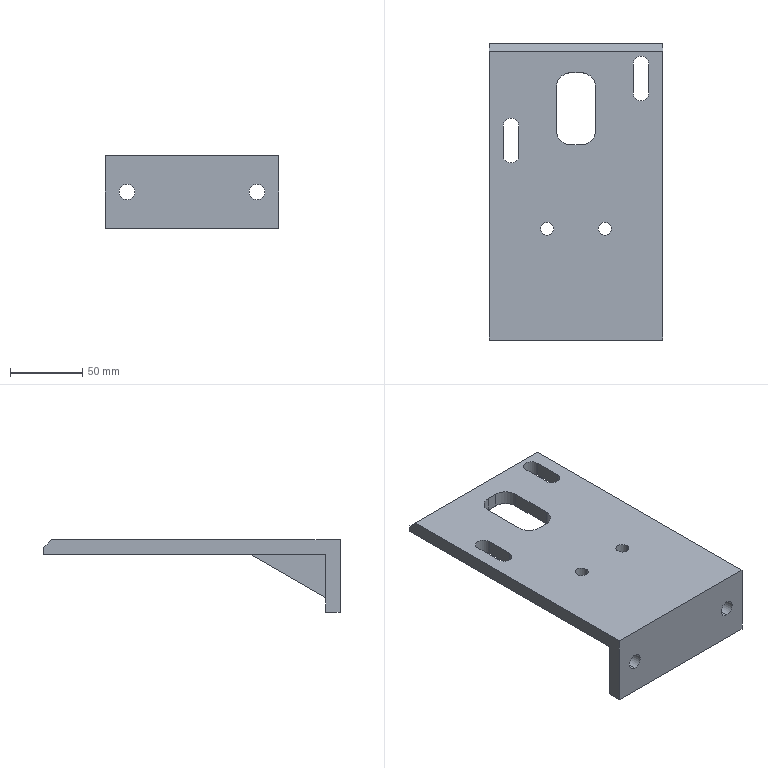Part | 1 solid | 39 faces | box 120 x 205 x 50 mm | volume 285973 mm3 | plane 23 | cylinder 16 | commonest cylinder face diameters 11 x8 9 x4 20 x4
STEP:
#1=CARTESIAN_POINT('',(60.,105.,-5.));
#2=VERTEX_POINT('',#1);
#3=CARTESIAN_POINT('',(60.,100.,0.));
#4=VERTEX_POINT('',#3);
#5=CARTESIAN_POINT('',(60.,100.,0.));
#6=DIRECTION('',(0.,-0.7071,0.7071));
#7=VECTOR('',#6,1000.);
#8=LINE('',#5,#7);
#9=EDGE_CURVE('',#2,#4,#8,.T.);
#10=ORIENTED_EDGE('',*,*,#9,.F.);
#11=CARTESIAN_POINT('',(-60.,105.,-5.));
#12=VERTEX_POINT('',#11);
#13=CARTESIAN_POINT('',(60.,105.,-5.));
#14=DIRECTION('',(1.,0.,0.));
#15=VECTOR('',#14,1000.);
#16=LINE('',#13,#15);
#17=EDGE_CURVE('',#12,#2,#16,.T.);
#18=ORIENTED_EDGE('',*,*,#17,.F.);
#19=CARTESIAN_POINT('',(-60.,100.,0.));
#20=VERTEX_POINT('',#19);
#21=CARTESIAN_POINT('',(-60.,0.,100.));
#22=DIRECTION('',(0.,0.7071,-0.7071));
#23=VECTOR('',#22,1000.);
#24=LINE('',#21,#23);
#25=EDGE_CURVE('',#20,#12,#24,.T.);
#26=ORIENTED_EDGE('',*,*,#25,.F.);
#27=CARTESIAN_POINT('',(60.,100.,0.));
#28=DIRECTION('',(-1.,0.,0.));
#29=VECTOR('',#28,1000.);
#30=LINE('',#27,#29);
#31=EDGE_CURVE('',#4,#20,#30,.T.);
#32=ORIENTED_EDGE('',*,*,#31,.F.);
#33=EDGE_LOOP('',(#10,#18,#26,#32));
#34=FACE_BOUND('',#33,.T.);
#35=CARTESIAN_POINT('',(60.,100.,0.));
#36=DIRECTION('',(0.,-0.7071,-0.7071));
#37=DIRECTION('',(0.,-0.7071,0.7071));
#38=AXIS2_PLACEMENT_3D('',#35,#36,#37);
#39=PLANE('',#38);
#40=ADVANCED_FACE('',(#34),#39,.F.);
#41=CARTESIAN_POINT('',(-15.,-38.038,-10.));
#42=VERTEX_POINT('',#41);
#43=CARTESIAN_POINT('',(-25.,-38.038,-10.));
#44=VERTEX_POINT('',#43);
#45=CARTESIAN_POINT('',(60.,-38.038,-10.));
#46=DIRECTION('',(-1.,0.,0.));
#47=VECTOR('',#46,1000.);
#48=LINE('',#45,#47);
#49=EDGE_CURVE('',#42,#44,#48,.T.);
#50=ORIENTED_EDGE('',*,*,#49,.F.);
#51=CARTESIAN_POINT('',(-15.,-90.,-40.));
#52=VERTEX_POINT('',#51);
#53=CARTESIAN_POINT('',(-15.,-90.,-40.));
#54=DIRECTION('',(0.,0.866,0.5));
#55=VECTOR('',#54,1000.);
#56=LINE('',#53,#55);
#57=EDGE_CURVE('',#52,#42,#56,.T.);
#58=ORIENTED_EDGE('',*,*,#57,.F.);
#59=CARTESIAN_POINT('',(-25.,-90.,-40.));
#60=VERTEX_POINT('',#59);
#61=CARTESIAN_POINT('',(60.,-90.,-40.));
#62=DIRECTION('',(1.,0.,0.));
#63=VECTOR('',#62,1000.);
#64=LINE('',#61,#63);
#65=EDGE_CURVE('',#60,#52,#64,.T.);
#66=ORIENTED_EDGE('',*,*,#65,.F.);
#67=CARTESIAN_POINT('',(-25.,-90.,-40.));
#68=DIRECTION('',(0.,0.866,0.5));
#69=VECTOR('',#68,1000.);
#70=LINE('',#67,#69);
#71=EDGE_CURVE('',#60,#44,#70,.T.);
#72=ORIENTED_EDGE('',*,*,#71,.T.);
#73=EDGE_LOOP('',(#50,#58,#66,#72));
#74=FACE_BOUND('',#73,.T.);
#75=CARTESIAN_POINT('',(-20.,-90.,-40.));
#76=DIRECTION('',(0.,-0.5,0.866));
#77=DIRECTION('',(1.,0.,0.));
#78=AXIS2_PLACEMENT_3D('',#75,#76,#77);
#79=PLANE('',#78);
#80=ADVANCED_FACE('',(#74),#79,.F.);
#81=ORIENTED_EDGE('',*,*,#57,.T.);
#82=CARTESIAN_POINT('',(-15.,-90.,-10.));
#83=VERTEX_POINT('',#82);
#84=CARTESIAN_POINT('',(-15.,-100.,-10.));
#85=DIRECTION('',(0.,-1.,0.));
#86=VECTOR('',#85,1000.);
#87=LINE('',#84,#86);
#88=EDGE_CURVE('',#42,#83,#87,.T.);
#89=ORIENTED_EDGE('',*,*,#88,.T.);
#90=CARTESIAN_POINT('',(-15.,-90.,-50.));
#91=DIRECTION('',(0.,0.,-1.));
#92=VECTOR('',#91,1000.);
#93=LINE('',#90,#92);
#94=EDGE_CURVE('',#83,#52,#93,.T.);
#95=ORIENTED_EDGE('',*,*,#94,.T.);
#96=EDGE_LOOP('',(#81,#89,#95));
#97=FACE_BOUND('',#96,.T.);
#98=CARTESIAN_POINT('',(-15.,2.5,-25.));
#99=DIRECTION('',(-1.,0.,0.));
#100=DIRECTION('',(0.,0.,-1.));
#101=AXIS2_PLACEMENT_3D('',#98,#99,#100);
#102=PLANE('',#101);
#103=ADVANCED_FACE('',(#97),#102,.F.);
#104=CARTESIAN_POINT('',(-25.,-90.,-10.));
#105=VERTEX_POINT('',#104);
#106=CARTESIAN_POINT('',(-25.,-100.,-10.));
#107=DIRECTION('',(0.,-1.,0.));
#108=VECTOR('',#107,1000.);
#109=LINE('',#106,#108);
#110=EDGE_CURVE('',#44,#105,#109,.T.);
#111=ORIENTED_EDGE('',*,*,#110,.F.);
#112=ORIENTED_EDGE('',*,*,#71,.F.);
#113=CARTESIAN_POINT('',(-25.,-90.,-50.));
#114=DIRECTION('',(0.,0.,-1.));
#115=VECTOR('',#114,1000.);
#116=LINE('',#113,#115);
#117=EDGE_CURVE('',#105,#60,#116,.T.);
#118=ORIENTED_EDGE('',*,*,#117,.F.);
#119=EDGE_LOOP('',(#111,#112,#118));
#120=FACE_BOUND('',#119,.T.);
#121=CARTESIAN_POINT('',(-25.,2.5,-25.));
#122=DIRECTION('',(-1.,0.,0.));
#123=DIRECTION('',(0.,0.,-1.));
#124=AXIS2_PLACEMENT_3D('',#121,#122,#123);
#125=PLANE('',#124);
#126=ADVANCED_FACE('',(#120),#125,.T.);
#127=CARTESIAN_POINT('',(25.,-38.038,-10.));
#128=VERTEX_POINT('',#127);
#129=CARTESIAN_POINT('',(15.,-38.038,-10.));
#130=VERTEX_POINT('',#129);
#131=CARTESIAN_POINT('',(60.,-38.038,-10.));
#132=DIRECTION('',(-1.,0.,0.));
#133=VECTOR('',#132,1000.);
#134=LINE('',#131,#133);
#135=EDGE_CURVE('',#128,#130,#134,.T.);
#136=ORIENTED_EDGE('',*,*,#135,.F.);
#137=CARTESIAN_POINT('',(25.,-90.,-40.));
#138=VERTEX_POINT('',#137);
#139=CARTESIAN_POINT('',(25.,-90.,-40.));
#140=DIRECTION('',(0.,0.866,0.5));
#141=VECTOR('',#140,1000.);
#142=LINE('',#139,#141);
#143=EDGE_CURVE('',#138,#128,#142,.T.);
#144=ORIENTED_EDGE('',*,*,#143,.F.);
#145=CARTESIAN_POINT('',(15.,-90.,-40.));
#146=VERTEX_POINT('',#145);
#147=CARTESIAN_POINT('',(60.,-90.,-40.));
#148=DIRECTION('',(1.,0.,0.));
#149=VECTOR('',#148,1000.);
#150=LINE('',#147,#149);
#151=EDGE_CURVE('',#146,#138,#150,.T.);
#152=ORIENTED_EDGE('',*,*,#151,.F.);
#153=CARTESIAN_POINT('',(15.,-90.,-40.));
#154=DIRECTION('',(0.,0.866,0.5));
#155=VECTOR('',#154,1000.);
#156=LINE('',#153,#155);
#157=EDGE_CURVE('',#146,#130,#156,.T.);
#158=ORIENTED_EDGE('',*,*,#157,.T.);
#159=EDGE_LOOP('',(#136,#144,#152,#158));
#160=FACE_BOUND('',#159,.T.);
#161=CARTESIAN_POINT('',(20.,-90.,-40.));
#162=DIRECTION('',(0.,0.5,-0.866));
#163=DIRECTION('',(1.,0.,0.));
#164=AXIS2_PLACEMENT_3D('',#161,#162,#163);
#165=PLANE('',#164);
#166=ADVANCED_FACE('',(#160),#165,.T.);
#167=CARTESIAN_POINT('',(15.,-90.,-10.));
#168=VERTEX_POINT('',#167);
#169=CARTESIAN_POINT('',(15.,-90.,-50.));
#170=DIRECTION('',(0.,0.,1.));
#171=VECTOR('',#170,1000.);
#172=LINE('',#169,#171);
#173=EDGE_CURVE('',#146,#168,#172,.T.);
#174=ORIENTED_EDGE('',*,*,#173,.T.);
#175=CARTESIAN_POINT('',(15.,-100.,-10.));
#176=DIRECTION('',(0.,1.,0.));
#177=VECTOR('',#176,1000.);
#178=LINE('',#175,#177);
#179=EDGE_CURVE('',#168,#130,#178,.T.);
#180=ORIENTED_EDGE('',*,*,#179,.T.);
#181=ORIENTED_EDGE('',*,*,#157,.F.);
#182=EDGE_LOOP('',(#174,#180,#181));
#183=FACE_BOUND('',#182,.T.);
#184=CARTESIAN_POINT('',(15.,2.5,-25.));
#185=DIRECTION('',(1.,0.,0.));
#186=DIRECTION('',(0.,-1.,0.));
#187=AXIS2_PLACEMENT_3D('',#184,#185,#186);
#188=PLANE('',#187);
#189=ADVANCED_FACE('',(#183),#188,.F.);
#190=CARTESIAN_POINT('',(25.,-90.,-10.));
#191=VERTEX_POINT('',#190);
#192=CARTESIAN_POINT('',(25.,-100.,-10.));
#193=DIRECTION('',(0.,1.,0.));
#194=VECTOR('',#193,1000.);
#195=LINE('',#192,#194);
#196=EDGE_CURVE('',#191,#128,#195,.T.);
#197=ORIENTED_EDGE('',*,*,#196,.F.);
#198=CARTESIAN_POINT('',(25.,-90.,-50.));
#199=DIRECTION('',(0.,0.,1.));
#200=VECTOR('',#199,1000.);
#201=LINE('',#198,#200);
#202=EDGE_CURVE('',#138,#191,#201,.T.);
#203=ORIENTED_EDGE('',*,*,#202,.F.);
#204=ORIENTED_EDGE('',*,*,#143,.T.);
#205=EDGE_LOOP('',(#197,#203,#204));
#206=FACE_BOUND('',#205,.T.);
#207=CARTESIAN_POINT('',(25.,2.5,-25.));
#208=DIRECTION('',(1.,0.,0.));
#209=DIRECTION('',(0.,-1.,0.));
#210=AXIS2_PLACEMENT_3D('',#207,#208,#209);
#211=PLANE('',#210);
#212=ADVANCED_FACE('',(#206),#211,.T.);
#213=CARTESIAN_POINT('',(24.5,-23.,0.));
#214=VERTEX_POINT('',#213);
#215=CARTESIAN_POINT('',(24.5,-23.,-10.));
#216=VERTEX_POINT('',#215);
#217=CARTESIAN_POINT('',(24.5,-23.,-10.));
#218=DIRECTION('',(0.,0.,-1.));
#219=VECTOR('',#218,1000.);
#220=LINE('',#217,#219);
#221=EDGE_CURVE('',#214,#216,#220,.T.);
#222=ORIENTED_EDGE('',*,*,#221,.F.);
#223=CARTESIAN_POINT('',(15.5,-23.,0.));
#224=VERTEX_POINT('',#223);
#225=CARTESIAN_POINT('',(20.,-23.,0.));
#226=DIRECTION('',(0.,0.,-1.));
#227=DIRECTION('',(-1.,0.,0.));
#228=AXIS2_PLACEMENT_3D('',#225,#226,#227);
#229=CIRCLE('',#228,4.5);
#230=EDGE_CURVE('',#224,#214,#229,.T.);
#231=ORIENTED_EDGE('',*,*,#230,.F.);
#232=CARTESIAN_POINT('',(15.5,-23.,-10.));
#233=VERTEX_POINT('',#232);
#234=CARTESIAN_POINT('',(15.5,-23.,-10.));
#235=DIRECTION('',(0.,0.,-1.));
#236=VECTOR('',#235,1000.);
#237=LINE('',#234,#236);
#238=EDGE_CURVE('',#224,#233,#237,.T.);
#239=ORIENTED_EDGE('',*,*,#238,.T.);
#240=CARTESIAN_POINT('',(20.,-23.,-10.));
#241=DIRECTION('',(0.,0.,-1.));
#242=DIRECTION('',(-1.,0.,0.));
#243=AXIS2_PLACEMENT_3D('',#240,#241,#242);
#244=CIRCLE('',#243,4.5);
#245=EDGE_CURVE('',#233,#216,#244,.T.);
#246=ORIENTED_EDGE('',*,*,#245,.T.);
#247=EDGE_LOOP('',(#222,#231,#239,#246));
#248=FACE_BOUND('',#247,.T.);
#249=CARTESIAN_POINT('',(20.,-23.,-10.));
#250=DIRECTION('',(0.,0.,-1.));
#251=DIRECTION('',(1.,0.,0.));
#252=AXIS2_PLACEMENT_3D('',#249,#250,#251);
#253=CYLINDRICAL_SURFACE('',#252,4.5);
#254=ADVANCED_FACE('',(#248),#253,.F.);
#255=CARTESIAN_POINT('',(-15.5,-23.,0.));
#256=VERTEX_POINT('',#255);
#257=CARTESIAN_POINT('',(-15.5,-23.,-10.));
#258=VERTEX_POINT('',#257);
#259=CARTESIAN_POINT('',(-15.5,-23.,-10.));
#260=DIRECTION('',(0.,0.,-1.));
#261=VECTOR('',#260,1000.);
#262=LINE('',#259,#261);
#263=EDGE_CURVE('',#256,#258,#262,.T.);
#264=ORIENTED_EDGE('',*,*,#263,.F.);
#265=CARTESIAN_POINT('',(-24.5,-23.,0.));
#266=VERTEX_POINT('',#265);
#267=CARTESIAN_POINT('',(-20.,-23.,0.));
#268=DIRECTION('',(0.,0.,-1.));
#269=DIRECTION('',(-1.,0.,0.));
#270=AXIS2_PLACEMENT_3D('',#267,#268,#269);
#271=CIRCLE('',#270,4.5);
#272=EDGE_CURVE('',#266,#256,#271,.T.);
#273=ORIENTED_EDGE('',*,*,#272,.F.);
#274=CARTESIAN_POINT('',(-24.5,-23.,-10.));
#275=VERTEX_POINT('',#274);
#276=CARTESIAN_POINT('',(-24.5,-23.,-10.));
#277=DIRECTION('',(0.,0.,-1.));
#278=VECTOR('',#277,1000.);
#279=LINE('',#276,#278);
#280=EDGE_CURVE('',#266,#275,#279,.T.);
#281=ORIENTED_EDGE('',*,*,#280,.T.);
#282=CARTESIAN_POINT('',(-20.,-23.,-10.));
#283=DIRECTION('',(0.,0.,-1.));
#284=DIRECTION('',(-1.,0.,0.));
#285=AXIS2_PLACEMENT_3D('',#282,#283,#284);
#286=CIRCLE('',#285,4.5);
#287=EDGE_CURVE('',#275,#258,#286,.T.);
#288=ORIENTED_EDGE('',*,*,#287,.T.);
#289=EDGE_LOOP('',(#264,#273,#281,#288));
#290=FACE_BOUND('',#289,.T.);
#291=CARTESIAN_POINT('',(-20.,-23.,-10.));
#292=DIRECTION('',(0.,0.,-1.));
#293=DIRECTION('',(1.,0.,0.));
#294=AXIS2_PLACEMENT_3D('',#291,#292,#293);
#295=CYLINDRICAL_SURFACE('',#294,4.5);
#296=ADVANCED_FACE('',(#290),#295,.F.);
#297=CARTESIAN_POINT('',(-39.5,48.,-10.));
#298=VERTEX_POINT('',#297);
#299=CARTESIAN_POINT('',(-39.5,28.,-10.));
#300=VERTEX_POINT('',#299);
#301=CARTESIAN_POINT('',(-39.5,48.,-10.));
#302=DIRECTION('',(0.,-1.,0.));
#303=VECTOR('',#302,1000.);
#304=LINE('',#301,#303);
#305=EDGE_CURVE('',#298,#300,#304,.T.);
#306=ORIENTED_EDGE('',*,*,#305,.T.);
#307=CARTESIAN_POINT('',(-39.5,28.,0.));
#308=VERTEX_POINT('',#307);
#309=CARTESIAN_POINT('',(-39.5,28.,0.));
#310=DIRECTION('',(0.,0.,-1.));
#311=VECTOR('',#310,1000.);
#312=LINE('',#309,#311);
#313=EDGE_CURVE('',#308,#300,#312,.T.);
#314=ORIENTED_EDGE('',*,*,#313,.F.);
#315=CARTESIAN_POINT('',(-39.5,48.,0.));
#316=VERTEX_POINT('',#315);
#317=CARTESIAN_POINT('',(-39.5,48.,0.));
#318=DIRECTION('',(0.,-1.,0.));
#319=VECTOR('',#318,1000.);
#320=LINE('',#317,#319);
#321=EDGE_CURVE('',#316,#308,#320,.T.);
#322=ORIENTED_EDGE('',*,*,#321,.F.);
#323=CARTESIAN_POINT('',(-39.5,48.,0.));
#324=DIRECTION('',(0.,0.,-1.));
#325=VECTOR('',#324,1000.);
#326=LINE('',#323,#325);
#327=EDGE_CURVE('',#316,#298,#326,.T.);
#328=ORIENTED_EDGE('',*,*,#327,.T.);
#329=EDGE_LOOP('',(#306,#314,#322,#328));
#330=FACE_BOUND('',#329,.T.);
#331=CARTESIAN_POINT('',(-39.5,48.,0.));
#332=DIRECTION('',(1.,0.,0.));
#333=DIRECTION('',(0.,-1.,0.));
#334=AXIS2_PLACEMENT_3D('',#331,#332,#333);
#335=PLANE('',#334);
#336=ADVANCED_FACE('',(#330),#335,.F.);
#337=CARTESIAN_POINT('',(-50.5,28.,-10.));
#338=VERTEX_POINT('',#337);
#339=CARTESIAN_POINT('',(-45.,28.,-10.));
#340=DIRECTION('',(0.,0.,-1.));
#341=DIRECTION('',(-1.,0.,0.));
#342=AXIS2_PLACEMENT_3D('',#339,#340,#341);
#343=CIRCLE('',#342,5.5);
#344=EDGE_CURVE('',#300,#338,#343,.T.);
#345=ORIENTED_EDGE('',*,*,#344,.T.);
#346=CARTESIAN_POINT('',(-50.5,28.,0.));
#347=VERTEX_POINT('',#346);
#348=CARTESIAN_POINT('',(-50.5,28.,0.));
#349=DIRECTION('',(0.,0.,-1.));
#350=VECTOR('',#349,1000.);
#351=LINE('',#348,#350);
#352=EDGE_CURVE('',#347,#338,#351,.T.);
#353=ORIENTED_EDGE('',*,*,#352,.F.);
#354=CARTESIAN_POINT('',(-45.,28.,0.));
#355=DIRECTION('',(0.,0.,-1.));
#356=DIRECTION('',(-1.,0.,0.));
#357=AXIS2_PLACEMENT_3D('',#354,#355,#356);
#358=CIRCLE('',#357,5.5);
#359=EDGE_CURVE('',#308,#347,#358,.T.);
#360=ORIENTED_EDGE('',*,*,#359,.F.);
#361=ORIENTED_EDGE('',*,*,#313,.T.);
#362=EDGE_LOOP('',(#345,#353,#360,#361));
#363=FACE_BOUND('',#362,.T.);
#364=CARTESIAN_POINT('',(-45.,28.,0.));
#365=DIRECTION('',(0.,0.,-1.));
#366=DIRECTION('',(1.,0.,0.));
#367=AXIS2_PLACEMENT_3D('',#364,#365,#366);
#368=CYLINDRICAL_SURFACE('',#367,5.5);
#369=ADVANCED_FACE('',(#363),#368,.F.);
#370=CARTESIAN_POINT('',(-50.5,48.,-10.));
#371=VERTEX_POINT('',#370);
#372=CARTESIAN_POINT('',(-50.5,48.,-10.));
#373=DIRECTION('',(0.,1.,0.));
#374=VECTOR('',#373,1000.);
#375=LINE('',#372,#374);
#376=EDGE_CURVE('',#338,#371,#375,.T.);
#377=ORIENTED_EDGE('',*,*,#376,.T.);
#378=CARTESIAN_POINT('',(-50.5,48.,0.));
#379=VERTEX_POINT('',#378);
#380=CARTESIAN_POINT('',(-50.5,48.,0.));
#381=DIRECTION('',(0.,0.,-1.));
#382=VECTOR('',#381,1000.);
#383=LINE('',#380,#382);
#384=EDGE_CURVE('',#379,#371,#383,.T.);
#385=ORIENTED_EDGE('',*,*,#384,.F.);
#386=CARTESIAN_POINT('',(-50.5,48.,0.));
#387=DIRECTION('',(0.,1.,0.));
#388=VECTOR('',#387,1000.);
#389=LINE('',#386,#388);
#390=EDGE_CURVE('',#347,#379,#389,.T.);
#391=ORIENTED_EDGE('',*,*,#390,.F.);
#392=ORIENTED_EDGE('',*,*,#352,.T.);
#393=EDGE_LOOP('',(#377,#385,#391,#392));
#394=FACE_BOUND('',#393,.T.);
#395=CARTESIAN_POINT('',(-50.5,48.,0.));
#396=DIRECTION('',(-1.,0.,0.));
#397=DIRECTION('',(0.,0.,-1.));
#398=AXIS2_PLACEMENT_3D('',#395,#396,#397);
#399=PLANE('',#398);
#400=ADVANCED_FACE('',(#394),#399,.F.);
#401=CARTESIAN_POINT('',(-45.,48.,-10.));
#402=DIRECTION('',(0.,0.,-1.));
#403=DIRECTION('',(-1.,0.,0.));
#404=AXIS2_PLACEMENT_3D('',#401,#402,#403);
#405=CIRCLE('',#404,5.5);
#406=EDGE_CURVE('',#371,#298,#405,.T.);
#407=ORIENTED_EDGE('',*,*,#406,.T.);
#408=ORIENTED_EDGE('',*,*,#327,.F.);
#409=CARTESIAN_POINT('',(-45.,48.,0.));
#410=DIRECTION('',(0.,0.,-1.));
#411=DIRECTION('',(-1.,0.,0.));
#412=AXIS2_PLACEMENT_3D('',#409,#410,#411);
#413=CIRCLE('',#412,5.5);
#414=EDGE_CURVE('',#379,#316,#413,.T.);
#415=ORIENTED_EDGE('',*,*,#414,.F.);
#416=ORIENTED_EDGE('',*,*,#384,.T.);
#417=EDGE_LOOP('',(#407,#408,#415,#416));
#418=FACE_BOUND('',#417,.T.);
#419=CARTESIAN_POINT('',(-45.,48.,0.));
#420=DIRECTION('',(0.,0.,-1.));
#421=DIRECTION('',(1.,0.,0.));
#422=AXIS2_PLACEMENT_3D('',#419,#420,#421);
#423=CYLINDRICAL_SURFACE('',#422,5.5);
#424=ADVANCED_FACE('',(#418),#423,.F.);
#425=CARTESIAN_POINT('',(50.5,91.,-10.));
#426=VERTEX_POINT('',#425);
#427=CARTESIAN_POINT('',(50.5,71.,-10.));
#428=VERTEX_POINT('',#427);
#429=CARTESIAN_POINT('',(50.5,91.,-10.));
#430=DIRECTION('',(0.,-1.,0.));
#431=VECTOR('',#430,1000.);
#432=LINE('',#429,#431);
#433=EDGE_CURVE('',#426,#428,#432,.T.);
#434=ORIENTED_EDGE('',*,*,#433,.T.);
#435=CARTESIAN_POINT('',(50.5,71.,0.));
#436=VERTEX_POINT('',#435);
#437=CARTESIAN_POINT('',(50.5,71.,0.));
#438=DIRECTION('',(0.,0.,-1.));
#439=VECTOR('',#438,1000.);
#440=LINE('',#437,#439);
#441=EDGE_CURVE('',#436,#428,#440,.T.);
#442=ORIENTED_EDGE('',*,*,#441,.F.);
#443=CARTESIAN_POINT('',(50.5,91.,0.));
#444=VERTEX_POINT('',#443);
#445=CARTESIAN_POINT('',(50.5,91.,0.));
#446=DIRECTION('',(0.,-1.,0.));
#447=VECTOR('',#446,1000.);
#448=LINE('',#445,#447);
#449=EDGE_CURVE('',#444,#436,#448,.T.);
#450=ORIENTED_EDGE('',*,*,#449,.F.);
#451=CARTESIAN_POINT('',(50.5,91.,0.));
#452=DIRECTION('',(0.,0.,-1.));
#453=VECTOR('',#452,1000.);
#454=LINE('',#451,#453);
#455=EDGE_CURVE('',#444,#426,#454,.T.);
#456=ORIENTED_EDGE('',*,*,#455,.T.);
#457=EDGE_LOOP('',(#434,#442,#450,#456));
#458=FACE_BOUND('',#457,.T.);
#459=CARTESIAN_POINT('',(50.5,91.,0.));
#460=DIRECTION('',(1.,0.,0.));
#461=DIRECTION('',(0.,-1.,0.));
#462=AXIS2_PLACEMENT_3D('',#459,#460,#461);
#463=PLANE('',#462);
#464=ADVANCED_FACE('',(#458),#463,.F.);
#465=CARTESIAN_POINT('',(39.5,71.,-10.));
#466=VERTEX_POINT('',#465);
#467=CARTESIAN_POINT('',(45.,71.,-10.));
#468=DIRECTION('',(0.,0.,-1.));
#469=DIRECTION('',(-1.,0.,0.));
#470=AXIS2_PLACEMENT_3D('',#467,#468,#469);
#471=CIRCLE('',#470,5.5);
#472=EDGE_CURVE('',#428,#466,#471,.T.);
#473=ORIENTED_EDGE('',*,*,#472,.T.);
#474=CARTESIAN_POINT('',(39.5,71.,0.));
#475=VERTEX_POINT('',#474);
#476=CARTESIAN_POINT('',(39.5,71.,0.));
#477=DIRECTION('',(0.,0.,-1.));
#478=VECTOR('',#477,1000.);
#479=LINE('',#476,#478);
#480=EDGE_CURVE('',#475,#466,#479,.T.);
#481=ORIENTED_EDGE('',*,*,#480,.F.);
#482=CARTESIAN_POINT('',(45.,71.,0.));
#483=DIRECTION('',(0.,0.,-1.));
#484=DIRECTION('',(-1.,0.,0.));
#485=AXIS2_PLACEMENT_3D('',#482,#483,#484);
#486=CIRCLE('',#485,5.5);
#487=EDGE_CURVE('',#436,#475,#486,.T.);
#488=ORIENTED_EDGE('',*,*,#487,.F.);
#489=ORIENTED_EDGE('',*,*,#441,.T.);
#490=EDGE_LOOP('',(#473,#481,#488,#489));
#491=FACE_BOUND('',#490,.T.);
#492=CARTESIAN_POINT('',(45.,71.,0.));
#493=DIRECTION('',(0.,0.,-1.));
#494=DIRECTION('',(1.,0.,0.));
#495=AXIS2_PLACEMENT_3D('',#492,#493,#494);
#496=CYLINDRICAL_SURFACE('',#495,5.5);
#497=ADVANCED_FACE('',(#491),#496,.F.);
#498=CARTESIAN_POINT('',(39.5,91.,-10.));
#499=VERTEX_POINT('',#498);
#500=CARTESIAN_POINT('',(39.5,91.,-10.));
#501=DIRECTION('',(0.,1.,0.));
#502=VECTOR('',#501,1000.);
#503=LINE('',#500,#502);
#504=EDGE_CURVE('',#466,#499,#503,.T.);
#505=ORIENTED_EDGE('',*,*,#504,.T.);
#506=CARTESIAN_POINT('',(39.5,91.,0.));
#507=VERTEX_POINT('',#506);
#508=CARTESIAN_POINT('',(39.5,91.,0.));
#509=DIRECTION('',(0.,0.,-1.));
#510=VECTOR('',#509,1000.);
#511=LINE('',#508,#510);
#512=EDGE_CURVE('',#507,#499,#511,.T.);
#513=ORIENTED_EDGE('',*,*,#512,.F.);
#514=CARTESIAN_POINT('',(39.5,91.,0.));
#515=DIRECTION('',(0.,1.,0.));
#516=VECTOR('',#515,1000.);
#517=LINE('',#514,#516);
#518=EDGE_CURVE('',#475,#507,#517,.T.);
#519=ORIENTED_EDGE('',*,*,#518,.F.);
#520=ORIENTED_EDGE('',*,*,#480,.T.);
#521=EDGE_LOOP('',(#505,#513,#519,#520));
#522=FACE_BOUND('',#521,.T.);
#523=CARTESIAN_POINT('',(39.5,91.,0.));
#524=DIRECTION('',(-1.,0.,0.));
#525=DIRECTION('',(0.,0.,-1.));
#526=AXIS2_PLACEMENT_3D('',#523,#524,#525);
#527=PLANE('',#526);
#528=ADVANCED_FACE('',(#522),#527,.F.);
#529=CARTESIAN_POINT('',(45.,91.,-10.));
#530=DIRECTION('',(0.,0.,-1.));
#531=DIRECTION('',(-1.,0.,0.));
#532=AXIS2_PLACEMENT_3D('',#529,#530,#531);
#533=CIRCLE('',#532,5.5);
#534=EDGE_CURVE('',#499,#426,#533,.T.);
#535=ORIENTED_EDGE('',*,*,#534,.T.);
#536=ORIENTED_EDGE('',*,*,#455,.F.);
#537=CARTESIAN_POINT('',(45.,91.,0.));
#538=DIRECTION('',(0.,0.,-1.));
#539=DIRECTION('',(-1.,0.,0.));
#540=AXIS2_PLACEMENT_3D('',#537,#538,#539);
#541=CIRCLE('',#540,5.5);
#542=EDGE_CURVE('',#507,#444,#541,.T.);
#543=ORIENTED_EDGE('',*,*,#542,.F.);
#544=ORIENTED_EDGE('',*,*,#512,.T.);
#545=EDGE_LOOP('',(#535,#536,#543,#544));
#546=FACE_BOUND('',#545,.T.);
#547=CARTESIAN_POINT('',(45.,91.,0.));
#548=DIRECTION('',(0.,0.,-1.));
#549=DIRECTION('',(1.,0.,0.));
#550=AXIS2_PLACEMENT_3D('',#547,#548,#549);
#551=CYLINDRICAL_SURFACE('',#550,5.5);
#552=ADVANCED_FACE('',(#546),#551,.F.);
#553=CARTESIAN_POINT('',(-3.5,35.,0.));
#554=VERTEX_POINT('',#553);
#555=CARTESIAN_POINT('',(-13.5,45.,0.));
#556=VERTEX_POINT('',#555);
#557=CARTESIAN_POINT('',(-3.5,45.,0.));
#558=DIRECTION('',(0.,0.,-1.));
#559=DIRECTION('',(1.,0.,0.));
#560=AXIS2_PLACEMENT_3D('',#557,#558,#559);
#561=CIRCLE('',#560,10.);
#562=EDGE_CURVE('',#554,#556,#561,.T.);
#563=ORIENTED_EDGE('',*,*,#562,.F.);
#564=CARTESIAN_POINT('',(-3.5,35.,-10.));
#565=VERTEX_POINT('',#564);
#566=CARTESIAN_POINT('',(-3.5,35.,0.));
#567=DIRECTION('',(0.,0.,1.));
#568=VECTOR('',#567,1000.);
#569=LINE('',#566,#568);
#570=EDGE_CURVE('',#565,#554,#569,.T.);
#571=ORIENTED_EDGE('',*,*,#570,.F.);
#572=CARTESIAN_POINT('',(-13.5,45.,-10.));
#573=VERTEX_POINT('',#572);
#574=CARTESIAN_POINT('',(-3.5,45.,-10.));
#575=DIRECTION('',(0.,0.,1.));
#576=DIRECTION('',(1.,0.,0.));
#577=AXIS2_PLACEMENT_3D('',#574,#575,#576);
#578=CIRCLE('',#577,10.);
#579=EDGE_CURVE('',#573,#565,#578,.T.);
#580=ORIENTED_EDGE('',*,*,#579,.F.);
#581=CARTESIAN_POINT('',(-13.5,45.,-10.));
#582=DIRECTION('',(0.,0.,-1.));
#583=VECTOR('',#582,1000.);
#584=LINE('',#581,#583);
#585=EDGE_CURVE('',#556,#573,#584,.T.);
#586=ORIENTED_EDGE('',*,*,#585,.F.);
#587=EDGE_LOOP('',(#563,#571,#580,#586));
#588=FACE_BOUND('',#587,.T.);
#589=CARTESIAN_POINT('',(-3.5,45.,0.));
#590=DIRECTION('',(0.,0.,1.));
#591=DIRECTION('',(-1.,0.,0.));
#592=AXIS2_PLACEMENT_3D('',#589,#590,#591);
#593=CYLINDRICAL_SURFACE('',#592,10.);
#594=ADVANCED_FACE('',(#588),#593,.F.);
#595=CARTESIAN_POINT('',(-13.5,75.,0.));
#596=VERTEX_POINT('',#595);
#597=CARTESIAN_POINT('',(-3.5,85.,0.));
#598=VERTEX_POINT('',#597);
#599=CARTESIAN_POINT('',(-3.5,75.,0.));
#600=DIRECTION('',(0.,0.,-1.));
#601=DIRECTION('',(1.,0.,0.));
#602=AXIS2_PLACEMENT_3D('',#599,#600,#601);
#603=CIRCLE('',#602,10.);
#604=EDGE_CURVE('',#596,#598,#603,.T.);
#605=ORIENTED_EDGE('',*,*,#604,.F.);
#606=CARTESIAN_POINT('',(-13.5,75.,-10.));
#607=VERTEX_POINT('',#606);
#608=CARTESIAN_POINT('',(-13.5,75.,0.));
#609=DIRECTION('',(0.,0.,1.));
#610=VECTOR('',#609,1000.);
#611=LINE('',#608,#610);
#612=EDGE_CURVE('',#607,#596,#611,.T.);
#613=ORIENTED_EDGE('',*,*,#612,.F.);
#614=CARTESIAN_POINT('',(-3.5,85.,-10.));
#615=VERTEX_POINT('',#614);
#616=CARTESIAN_POINT('',(-3.5,75.,-10.));
#617=DIRECTION('',(0.,0.,1.));
#618=DIRECTION('',(1.,0.,0.));
#619=AXIS2_PLACEMENT_3D('',#616,#617,#618);
#620=CIRCLE('',#619,10.);
#621=EDGE_CURVE('',#615,#607,#620,.T.);
#622=ORIENTED_EDGE('',*,*,#621,.F.);
#623=CARTESIAN_POINT('',(-3.5,85.,-10.));
#624=DIRECTION('',(0.,0.,-1.));
#625=VECTOR('',#624,1000.);
#626=LINE('',#623,#625);
#627=EDGE_CURVE('',#598,#615,#626,.T.);
#628=ORIENTED_EDGE('',*,*,#627,.F.);
#629=EDGE_LOOP('',(#605,#613,#622,#628));
#630=FACE_BOUND('',#629,.T.);
#631=CARTESIAN_POINT('',(-3.5,75.,0.));
#632=DIRECTION('',(0.,0.,1.));
#633=DIRECTION('',(-1.,0.,0.));
#634=AXIS2_PLACEMENT_3D('',#631,#632,#633);
#635=CYLINDRICAL_SURFACE('',#634,10.);
#636=ADVANCED_FACE('',(#630),#635,.F.);
#637=CARTESIAN_POINT('',(3.5,85.,0.));
#638=VERTEX_POINT('',#637);
#639=CARTESIAN_POINT('',(13.5,75.,0.));
#640=VERTEX_POINT('',#639);
#641=CARTESIAN_POINT('',(3.5,75.,0.));
#642=DIRECTION('',(0.,0.,-1.));
#643=DIRECTION('',(1.,0.,0.));
#644=AXIS2_PLACEMENT_3D('',#641,#642,#643);
#645=CIRCLE('',#644,10.);
#646=EDGE_CURVE('',#638,#640,#645,.T.);
#647=ORIENTED_EDGE('',*,*,#646,.F.);
#648=CARTESIAN_POINT('',(3.5,85.,-10.));
#649=VERTEX_POINT('',#648);
#650=CARTESIAN_POINT('',(3.5,85.,0.));
#651=DIRECTION('',(0.,0.,1.));
#652=VECTOR('',#651,1000.);
#653=LINE('',#650,#652);
#654=EDGE_CURVE('',#649,#638,#653,.T.);
#655=ORIENTED_EDGE('',*,*,#654,.F.);
#656=CARTESIAN_POINT('',(13.5,75.,-10.));
#657=VERTEX_POINT('',#656);
#658=CARTESIAN_POINT('',(3.5,75.,-10.));
#659=DIRECTION('',(0.,0.,1.));
#660=DIRECTION('',(1.,0.,0.));
#661=AXIS2_PLACEMENT_3D('',#658,#659,#660);
#662=CIRCLE('',#661,10.);
#663=EDGE_CURVE('',#657,#649,#662,.T.);
#664=ORIENTED_EDGE('',*,*,#663,.F.);
#665=CARTESIAN_POINT('',(13.5,75.,-10.));
#666=DIRECTION('',(0.,0.,-1.));
#667=VECTOR('',#666,1000.);
#668=LINE('',#665,#667);
#669=EDGE_CURVE('',#640,#657,#668,.T.);
#670=ORIENTED_EDGE('',*,*,#669,.F.);
#671=EDGE_LOOP('',(#647,#655,#664,#670));
#672=FACE_BOUND('',#671,.T.);
#673=CARTESIAN_POINT('',(3.5,75.,0.));
#674=DIRECTION('',(0.,0.,1.));
#675=DIRECTION('',(-1.,0.,0.));
#676=AXIS2_PLACEMENT_3D('',#673,#674,#675);
#677=CYLINDRICAL_SURFACE('',#676,10.);
#678=ADVANCED_FACE('',(#672),#677,.F.);
#679=CARTESIAN_POINT('',(13.5,45.,0.));
#680=VERTEX_POINT('',#679);
#681=CARTESIAN_POINT('',(3.5,35.,0.));
#682=VERTEX_POINT('',#681);
#683=CARTESIAN_POINT('',(3.5,45.,0.));
#684=DIRECTION('',(0.,0.,-1.));
#685=DIRECTION('',(1.,0.,0.));
#686=AXIS2_PLACEMENT_3D('',#683,#684,#685);
#687=CIRCLE('',#686,10.);
#688=EDGE_CURVE('',#680,#682,#687,.T.);
#689=ORIENTED_EDGE('',*,*,#688,.F.);
#690=CARTESIAN_POINT('',(13.5,45.,-10.));
#691=VERTEX_POINT('',#690);
#692=CARTESIAN_POINT('',(13.5,45.,0.));
#693=DIRECTION('',(0.,0.,1.));
#694=VECTOR('',#693,1000.);
#695=LINE('',#692,#694);
#696=EDGE_CURVE('',#691,#680,#695,.T.);
#697=ORIENTED_EDGE('',*,*,#696,.F.);
#698=CARTESIAN_POINT('',(3.5,35.,-10.));
#699=VERTEX_POINT('',#698);
#700=CARTESIAN_POINT('',(3.5,45.,-10.));
#701=DIRECTION('',(0.,0.,1.));
#702=DIRECTION('',(1.,0.,0.));
#703=AXIS2_PLACEMENT_3D('',#700,#701,#702);
#704=CIRCLE('',#703,10.);
#705=EDGE_CURVE('',#699,#691,#704,.T.);
#706=ORIENTED_EDGE('',*,*,#705,.F.);
#707=CARTESIAN_POINT('',(3.5,35.,-10.));
#708=DIRECTION('',(0.,0.,-1.));
#709=VECTOR('',#708,1000.);
#710=LINE('',#707,#709);
#711=EDGE_CURVE('',#682,#699,#710,.T.);
#712=ORIENTED_EDGE('',*,*,#711,.F.);
#713=EDGE_LOOP('',(#689,#697,#706,#712));
#714=FACE_BOUND('',#713,.T.);
#715=CARTESIAN_POINT('',(3.5,45.,0.));
#716=DIRECTION('',(0.,0.,1.));
#717=DIRECTION('',(-1.,0.,0.));
#718=AXIS2_PLACEMENT_3D('',#715,#716,#717);
#719=CYLINDRICAL_SURFACE('',#718,10.);
#720=ADVANCED_FACE('',(#714),#719,.F.);
#721=CARTESIAN_POINT('',(13.5,85.,-10.));
#722=DIRECTION('',(1.,0.,0.));
#723=VECTOR('',#722,1000.);
#724=LINE('',#721,#723);
#725=EDGE_CURVE('',#615,#649,#724,.T.);
#726=ORIENTED_EDGE('',*,*,#725,.T.);
#727=ORIENTED_EDGE('',*,*,#654,.T.);
#728=CARTESIAN_POINT('',(13.5,85.,0.));
#729=DIRECTION('',(1.,0.,0.));
#730=VECTOR('',#729,1000.);
#731=LINE('',#728,#730);
#732=EDGE_CURVE('',#598,#638,#731,.T.);
#733=ORIENTED_EDGE('',*,*,#732,.F.);
#734=ORIENTED_EDGE('',*,*,#627,.T.);
#735=EDGE_LOOP('',(#726,#727,#733,#734));
#736=FACE_BOUND('',#735,.T.);
#737=CARTESIAN_POINT('',(13.5,85.,0.));
#738=DIRECTION('',(0.,1.,0.));
#739=DIRECTION('',(-1.,0.,0.));
#740=AXIS2_PLACEMENT_3D('',#737,#738,#739);
#741=PLANE('',#740);
#742=ADVANCED_FACE('',(#736),#741,.F.);
#743=CARTESIAN_POINT('',(13.5,85.,-10.));
#744=DIRECTION('',(0.,-1.,0.));
#745=VECTOR('',#744,1000.);
#746=LINE('',#743,#745);
#747=EDGE_CURVE('',#657,#691,#746,.T.);
#748=ORIENTED_EDGE('',*,*,#747,.T.);
#749=ORIENTED_EDGE('',*,*,#696,.T.);
#750=CARTESIAN_POINT('',(13.5,85.,0.));
#751=DIRECTION('',(0.,-1.,0.));
#752=VECTOR('',#751,1000.);
#753=LINE('',#750,#752);
#754=EDGE_CURVE('',#640,#680,#753,.T.);
#755=ORIENTED_EDGE('',*,*,#754,.F.);
#756=ORIENTED_EDGE('',*,*,#669,.T.);
#757=EDGE_LOOP('',(#748,#749,#755,#756));
#758=FACE_BOUND('',#757,.T.);
#759=CARTESIAN_POINT('',(13.5,85.,0.));
#760=DIRECTION('',(1.,0.,0.));
#761=DIRECTION('',(0.,-1.,0.));
#762=AXIS2_PLACEMENT_3D('',#759,#760,#761);
#763=PLANE('',#762);
#764=ADVANCED_FACE('',(#758),#763,.F.);
#765=CARTESIAN_POINT('',(13.5,35.,0.));
#766=DIRECTION('',(-1.,0.,0.));
#767=VECTOR('',#766,1000.);
#768=LINE('',#765,#767);
#769=EDGE_CURVE('',#682,#554,#768,.T.);
#770=ORIENTED_EDGE('',*,*,#769,.F.);
#771=ORIENTED_EDGE('',*,*,#711,.T.);
#772=CARTESIAN_POINT('',(13.5,35.,-10.));
#773=DIRECTION('',(-1.,0.,0.));
#774=VECTOR('',#773,1000.);
#775=LINE('',#772,#774);
#776=EDGE_CURVE('',#699,#565,#775,.T.);
#777=ORIENTED_EDGE('',*,*,#776,.T.);
#778=ORIENTED_EDGE('',*,*,#570,.T.);
#779=EDGE_LOOP('',(#770,#771,#777,#778));
#780=FACE_BOUND('',#779,.T.);
#781=CARTESIAN_POINT('',(13.5,35.,0.));
#782=DIRECTION('',(0.,-1.,0.));
#783=DIRECTION('',(0.,0.,1.));
#784=AXIS2_PLACEMENT_3D('',#781,#782,#783);
#785=PLANE('',#784);
#786=ADVANCED_FACE('',(#780),#785,.F.);
#787=CARTESIAN_POINT('',(-13.5,85.,-10.));
#788=DIRECTION('',(0.,1.,0.));
#789=VECTOR('',#788,1000.);
#790=LINE('',#787,#789);
#791=EDGE_CURVE('',#573,#607,#790,.T.);
#792=ORIENTED_EDGE('',*,*,#791,.T.);
#793=ORIENTED_EDGE('',*,*,#612,.T.);
#794=CARTESIAN_POINT('',(-13.5,85.,0.));
#795=DIRECTION('',(0.,1.,0.));
#796=VECTOR('',#795,1000.);
#797=LINE('',#794,#796);
#798=EDGE_CURVE('',#556,#596,#797,.T.);
#799=ORIENTED_EDGE('',*,*,#798,.F.);
#800=ORIENTED_EDGE('',*,*,#585,.T.);
#801=EDGE_LOOP('',(#792,#793,#799,#800));
#802=FACE_BOUND('',#801,.T.);
#803=CARTESIAN_POINT('',(-13.5,85.,0.));
#804=DIRECTION('',(-1.,0.,0.));
#805=DIRECTION('',(0.,0.,-1.));
#806=AXIS2_PLACEMENT_3D('',#803,#804,#805);
#807=PLANE('',#806);
#808=ADVANCED_FACE('',(#802),#807,.F.);
#809=CARTESIAN_POINT('',(-45.,-100.,-30.5));
#810=VERTEX_POINT('',#809);
#811=CARTESIAN_POINT('',(-45.,-90.,-30.5));
#812=VERTEX_POINT('',#811);
#813=CARTESIAN_POINT('',(-45.,-90.,-30.5));
#814=DIRECTION('',(0.,1.,0.));
#815=VECTOR('',#814,1000.);
#816=LINE('',#813,#815);
#817=EDGE_CURVE('',#810,#812,#816,.T.);
#818=ORIENTED_EDGE('',*,*,#817,.F.);
#819=CARTESIAN_POINT('',(-45.,-100.,-19.5));
#820=VERTEX_POINT('',#819);
#821=CARTESIAN_POINT('',(-45.,-100.,-25.));
#822=DIRECTION('',(0.,1.,0.));
#823=DIRECTION('',(0.,0.,1.));
#824=AXIS2_PLACEMENT_3D('',#821,#822,#823);
#825=CIRCLE('',#824,5.5);
#826=EDGE_CURVE('',#820,#810,#825,.T.);
#827=ORIENTED_EDGE('',*,*,#826,.F.);
#828=CARTESIAN_POINT('',(-45.,-90.,-19.5));
#829=VERTEX_POINT('',#828);
#830=CARTESIAN_POINT('',(-45.,-90.,-19.5));
#831=DIRECTION('',(0.,1.,0.));
#832=VECTOR('',#831,1000.);
#833=LINE('',#830,#832);
#834=EDGE_CURVE('',#820,#829,#833,.T.);
#835=ORIENTED_EDGE('',*,*,#834,.T.);
#836=CARTESIAN_POINT('',(-45.,-90.,-25.));
#837=DIRECTION('',(0.,1.,0.));
#838=DIRECTION('',(0.,0.,1.));
#839=AXIS2_PLACEMENT_3D('',#836,#837,#838);
#840=CIRCLE('',#839,5.5);
#841=EDGE_CURVE('',#829,#812,#840,.T.);
#842=ORIENTED_EDGE('',*,*,#841,.T.);
#843=EDGE_LOOP('',(#818,#827,#835,#842));
#844=FACE_BOUND('',#843,.T.);
#845=CARTESIAN_POINT('',(-45.,-90.,-25.));
#846=DIRECTION('',(0.,1.,0.));
#847=DIRECTION('',(0.,0.,-1.));
#848=AXIS2_PLACEMENT_3D('',#845,#846,#847);
#849=CYLINDRICAL_SURFACE('',#848,5.5);
#850=ADVANCED_FACE('',(#844),#849,.F.);
#851=CARTESIAN_POINT('',(45.,-100.,-30.5));
#852=VERTEX_POINT('',#851);
#853=CARTESIAN_POINT('',(45.,-90.,-30.5));
#854=VERTEX_POINT('',#853);
#855=CARTESIAN_POINT('',(45.,-90.,-30.5));
#856=DIRECTION('',(0.,1.,0.));
#857=VECTOR('',#856,1000.);
#858=LINE('',#855,#857);
#859=EDGE_CURVE('',#852,#854,#858,.T.);
#860=ORIENTED_EDGE('',*,*,#859,.F.);
#861=CARTESIAN_POINT('',(45.,-100.,-19.5));
#862=VERTEX_POINT('',#861);
#863=CARTESIAN_POINT('',(45.,-100.,-25.));
#864=DIRECTION('',(0.,1.,0.));
#865=DIRECTION('',(0.,0.,1.));
#866=AXIS2_PLACEMENT_3D('',#863,#864,#865);
#867=CIRCLE('',#866,5.5);
#868=EDGE_CURVE('',#862,#852,#867,.T.);
#869=ORIENTED_EDGE('',*,*,#868,.F.);
#870=CARTESIAN_POINT('',(45.,-90.,-19.5));
#871=VERTEX_POINT('',#870);
#872=CARTESIAN_POINT('',(45.,-90.,-19.5));
#873=DIRECTION('',(0.,1.,0.));
#874=VECTOR('',#873,1000.);
#875=LINE('',#872,#874);
#876=EDGE_CURVE('',#862,#871,#875,.T.);
#877=ORIENTED_EDGE('',*,*,#876,.T.);
#878=CARTESIAN_POINT('',(45.,-90.,-25.));
#879=DIRECTION('',(0.,1.,0.));
#880=DIRECTION('',(0.,0.,1.));
#881=AXIS2_PLACEMENT_3D('',#878,#879,#880);
#882=CIRCLE('',#881,5.5);
#883=EDGE_CURVE('',#871,#854,#882,.T.);
#884=ORIENTED_EDGE('',*,*,#883,.T.);
#885=EDGE_LOOP('',(#860,#869,#877,#884));
#886=FACE_BOUND('',#885,.T.);
#887=CARTESIAN_POINT('',(45.,-90.,-25.));
#888=DIRECTION('',(0.,1.,0.));
#889=DIRECTION('',(0.,0.,-1.));
#890=AXIS2_PLACEMENT_3D('',#887,#888,#889);
#891=CYLINDRICAL_SURFACE('',#890,5.5);
#892=ADVANCED_FACE('',(#886),#891,.F.);
#893=CARTESIAN_POINT('',(-60.,-100.,0.));
#894=VERTEX_POINT('',#893);
#895=CARTESIAN_POINT('',(-60.,-100.,0.));
#896=DIRECTION('',(0.,1.,0.));
#897=VECTOR('',#896,1000.);
#898=LINE('',#895,#897);
#899=EDGE_CURVE('',#894,#20,#898,.T.);
#900=ORIENTED_EDGE('',*,*,#899,.T.);
#901=ORIENTED_EDGE('',*,*,#25,.T.);
#902=CARTESIAN_POINT('',(-60.,105.,-10.));
#903=VERTEX_POINT('',#902);
#904=CARTESIAN_POINT('',(-60.,105.,0.));
#905=DIRECTION('',(0.,0.,-1.));
#906=VECTOR('',#905,1000.);
#907=LINE('',#904,#906);
#908=EDGE_CURVE('',#12,#903,#907,.T.);
#909=ORIENTED_EDGE('',*,*,#908,.T.);
#910=CARTESIAN_POINT('',(-60.,-90.,-10.));
#911=VERTEX_POINT('',#910);
#912=CARTESIAN_POINT('',(-60.,-100.,-10.));
#913=DIRECTION('',(0.,1.,0.));
#914=VECTOR('',#913,1000.);
#915=LINE('',#912,#914);
#916=EDGE_CURVE('',#911,#903,#915,.T.);
#917=ORIENTED_EDGE('',*,*,#916,.F.);
#918=CARTESIAN_POINT('',(-60.,-90.,-50.));
#919=VERTEX_POINT('',#918);
#920=CARTESIAN_POINT('',(-60.,-90.,-50.));
#921=DIRECTION('',(0.,0.,1.));
#922=VECTOR('',#921,1000.);
#923=LINE('',#920,#922);
#924=EDGE_CURVE('',#919,#911,#923,.T.);
#925=ORIENTED_EDGE('',*,*,#924,.F.);
#926=CARTESIAN_POINT('',(-60.,-100.,-50.));
#927=VERTEX_POINT('',#926);
#928=CARTESIAN_POINT('',(-60.,-90.,-50.));
#929=DIRECTION('',(0.,-1.,0.));
#930=VECTOR('',#929,1000.);
#931=LINE('',#928,#930);
#932=EDGE_CURVE('',#919,#927,#931,.T.);
#933=ORIENTED_EDGE('',*,*,#932,.T.);
#934=CARTESIAN_POINT('',(-60.,-100.,-50.));
#935=DIRECTION('',(0.,0.,1.));
#936=VECTOR('',#935,1000.);
#937=LINE('',#934,#936);
#938=EDGE_CURVE('',#927,#894,#937,.T.);
#939=ORIENTED_EDGE('',*,*,#938,.T.);
#940=EDGE_LOOP('',(#900,#901,#909,#917,#925,#933,#939));
#941=FACE_BOUND('',#940,.T.);
#942=CARTESIAN_POINT('',(-60.,-100.,0.));
#943=DIRECTION('',(-1.,0.,0.));
#944=DIRECTION('',(0.,0.,-1.));
#945=AXIS2_PLACEMENT_3D('',#942,#943,#944);
#946=PLANE('',#945);
#947=ADVANCED_FACE('',(#941),#946,.T.);
#948=CARTESIAN_POINT('',(60.,105.,-10.));
#949=VERTEX_POINT('',#948);
#950=CARTESIAN_POINT('',(60.,105.,0.));
#951=DIRECTION('',(0.,0.,-1.));
#952=VECTOR('',#951,1000.);
#953=LINE('',#950,#952);
#954=EDGE_CURVE('',#2,#949,#953,.T.);
#955=ORIENTED_EDGE('',*,*,#954,.F.);
#956=ORIENTED_EDGE('',*,*,#9,.T.);
#957=CARTESIAN_POINT('',(60.,-100.,0.));
#958=VERTEX_POINT('',#957);
#959=CARTESIAN_POINT('',(60.,-100.,0.));
#960=DIRECTION('',(0.,1.,0.));
#961=VECTOR('',#960,1000.);
#962=LINE('',#959,#961);
#963=EDGE_CURVE('',#958,#4,#962,.T.);
#964=ORIENTED_EDGE('',*,*,#963,.F.);
#965=CARTESIAN_POINT('',(60.,-100.,-50.));
#966=VERTEX_POINT('',#965);
#967=CARTESIAN_POINT('',(60.,-100.,-50.));
#968=DIRECTION('',(0.,0.,1.));
#969=VECTOR('',#968,1000.);
#970=LINE('',#967,#969);
#971=EDGE_CURVE('',#966,#958,#970,.T.);
#972=ORIENTED_EDGE('',*,*,#971,.F.);
#973=CARTESIAN_POINT('',(60.,-90.,-50.));
#974=VERTEX_POINT('',#973);
#975=CARTESIAN_POINT('',(60.,-90.,-50.));
#976=DIRECTION('',(0.,-1.,0.));
#977=VECTOR('',#976,1000.);
#978=LINE('',#975,#977);
#979=EDGE_CURVE('',#974,#966,#978,.T.);
#980=ORIENTED_EDGE('',*,*,#979,.F.);
#981=CARTESIAN_POINT('',(60.,-90.,-10.));
#982=VERTEX_POINT('',#981);
#983=CARTESIAN_POINT('',(60.,-90.,-50.));
#984=DIRECTION('',(0.,0.,1.));
#985=VECTOR('',#984,1000.);
#986=LINE('',#983,#985);
#987=EDGE_CURVE('',#974,#982,#986,.T.);
#988=ORIENTED_EDGE('',*,*,#987,.T.);
#989=CARTESIAN_POINT('',(60.,-100.,-10.));
#990=DIRECTION('',(0.,1.,0.));
#991=VECTOR('',#990,1000.);
#992=LINE('',#989,#991);
#993=EDGE_CURVE('',#982,#949,#992,.T.);
#994=ORIENTED_EDGE('',*,*,#993,.T.);
#995=EDGE_LOOP('',(#955,#956,#964,#972,#980,#988,#994));
#996=FACE_BOUND('',#995,.T.);
#997=CARTESIAN_POINT('',(60.,-100.,0.));
#998=DIRECTION('',(-1.,0.,0.));
#999=DIRECTION('',(0.,0.,-1.));
#1000=AXIS2_PLACEMENT_3D('',#997,#998,#999);
#1001=PLANE('',#1000);
#1002=ADVANCED_FACE('',(#996),#1001,.F.);
#1003=ORIENTED_EDGE('',*,*,#883,.F.);
#1004=CARTESIAN_POINT('',(45.,-90.,-25.));
#1005=DIRECTION('',(0.,1.,0.));
#1006=DIRECTION('',(0.,0.,1.));
#1007=AXIS2_PLACEMENT_3D('',#1004,#1005,#1006);
#1008=CIRCLE('',#1007,5.5);
#1009=EDGE_CURVE('',#854,#871,#1008,.T.);
#1010=ORIENTED_EDGE('',*,*,#1009,.F.);
#1011=EDGE_LOOP('',(#1003,#1010));
#1012=FACE_BOUND('',#1011,.T.);
#1013=ORIENTED_EDGE('',*,*,#841,.F.);
#1014=CARTESIAN_POINT('',(-45.,-90.,-25.));
#1015=DIRECTION('',(0.,1.,0.));
#1016=DIRECTION('',(0.,0.,1.));
#1017=AXIS2_PLACEMENT_3D('',#1014,#1015,#1016);
#1018=CIRCLE('',#1017,5.5);
#1019=EDGE_CURVE('',#812,#829,#1018,.T.);
#1020=ORIENTED_EDGE('',*,*,#1019,.F.);
#1021=EDGE_LOOP('',(#1013,#1020));
#1022=FACE_BOUND('',#1021,.T.);
#1023=CARTESIAN_POINT('',(60.,-90.,-10.));
#1024=DIRECTION('',(-1.,0.,0.));
#1025=VECTOR('',#1024,1000.);
#1026=LINE('',#1023,#1025);
#1027=EDGE_CURVE('',#105,#911,#1026,.T.);
#1028=ORIENTED_EDGE('',*,*,#1027,.F.);
#1029=ORIENTED_EDGE('',*,*,#117,.T.);
#1030=ORIENTED_EDGE('',*,*,#65,.T.);
#1031=ORIENTED_EDGE('',*,*,#94,.F.);
#1032=CARTESIAN_POINT('',(60.,-90.,-10.));
#1033=DIRECTION('',(-1.,0.,0.));
#1034=VECTOR('',#1033,1000.);
#1035=LINE('',#1032,#1034);
#1036=EDGE_CURVE('',#168,#83,#1035,.T.);
#1037=ORIENTED_EDGE('',*,*,#1036,.F.);
#1038=ORIENTED_EDGE('',*,*,#173,.F.);
#1039=ORIENTED_EDGE('',*,*,#151,.T.);
#1040=ORIENTED_EDGE('',*,*,#202,.T.);
#1041=CARTESIAN_POINT('',(60.,-90.,-10.));
#1042=DIRECTION('',(-1.,0.,0.));
#1043=VECTOR('',#1042,1000.);
#1044=LINE('',#1041,#1043);
#1045=EDGE_CURVE('',#982,#191,#1044,.T.);
#1046=ORIENTED_EDGE('',*,*,#1045,.F.);
#1047=ORIENTED_EDGE('',*,*,#987,.F.);
#1048=CARTESIAN_POINT('',(60.,-90.,-50.));
#1049=DIRECTION('',(-1.,0.,0.));
#1050=VECTOR('',#1049,1000.);
#1051=LINE('',#1048,#1050);
#1052=EDGE_CURVE('',#974,#919,#1051,.T.);
#1053=ORIENTED_EDGE('',*,*,#1052,.T.);
#1054=ORIENTED_EDGE('',*,*,#924,.T.);
#1055=EDGE_LOOP('',(#1028,#1029,#1030,#1031,#1037,#1038,#1039,#1040,#1046,#1047,#1053,#1054));
#1056=FACE_BOUND('',#1055,.T.);
#1057=CARTESIAN_POINT('',(60.,-90.,-50.));
#1058=DIRECTION('',(0.,-1.,0.));
#1059=DIRECTION('',(0.,0.,1.));
#1060=AXIS2_PLACEMENT_3D('',#1057,#1058,#1059);
#1061=PLANE('',#1060);
#1062=ADVANCED_FACE('',(#1012,#1022,#1056),#1061,.F.);
#1063=ORIENTED_EDGE('',*,*,#932,.F.);
#1064=ORIENTED_EDGE('',*,*,#1052,.F.);
#1065=ORIENTED_EDGE('',*,*,#979,.T.);
#1066=CARTESIAN_POINT('',(60.,-100.,-50.));
#1067=DIRECTION('',(-1.,0.,0.));
#1068=VECTOR('',#1067,1000.);
#1069=LINE('',#1066,#1068);
#1070=EDGE_CURVE('',#966,#927,#1069,.T.);
#1071=ORIENTED_EDGE('',*,*,#1070,.T.);
#1072=EDGE_LOOP('',(#1063,#1064,#1065,#1071));
#1073=FACE_BOUND('',#1072,.T.);
#1074=CARTESIAN_POINT('',(60.,-90.,-50.));
#1075=DIRECTION('',(0.,0.,-1.));
#1076=DIRECTION('',(0.,1.,0.));
#1077=AXIS2_PLACEMENT_3D('',#1074,#1075,#1076);
#1078=PLANE('',#1077);
#1079=ADVANCED_FACE('',(#1073),#1078,.T.);
#1080=ORIENTED_EDGE('',*,*,#868,.T.);
#1081=CARTESIAN_POINT('',(45.,-100.,-25.));
#1082=DIRECTION('',(0.,1.,0.));
#1083=DIRECTION('',(0.,0.,1.));
#1084=AXIS2_PLACEMENT_3D('',#1081,#1082,#1083);
#1085=CIRCLE('',#1084,5.5);
#1086=EDGE_CURVE('',#852,#862,#1085,.T.);
#1087=ORIENTED_EDGE('',*,*,#1086,.T.);
#1088=EDGE_LOOP('',(#1080,#1087));
#1089=FACE_BOUND('',#1088,.T.);
#1090=ORIENTED_EDGE('',*,*,#826,.T.);
#1091=CARTESIAN_POINT('',(-45.,-100.,-25.));
#1092=DIRECTION('',(0.,1.,0.));
#1093=DIRECTION('',(0.,0.,1.));
#1094=AXIS2_PLACEMENT_3D('',#1091,#1092,#1093);
#1095=CIRCLE('',#1094,5.5);
#1096=EDGE_CURVE('',#810,#820,#1095,.T.);
#1097=ORIENTED_EDGE('',*,*,#1096,.T.);
#1098=EDGE_LOOP('',(#1090,#1097));
#1099=FACE_BOUND('',#1098,.T.);
#1100=CARTESIAN_POINT('',(60.,-100.,0.));
#1101=DIRECTION('',(-1.,0.,0.));
#1102=VECTOR('',#1101,1000.);
#1103=LINE('',#1100,#1102);
#1104=EDGE_CURVE('',#958,#894,#1103,.T.);
#1105=ORIENTED_EDGE('',*,*,#1104,.T.);
#1106=ORIENTED_EDGE('',*,*,#938,.F.);
#1107=ORIENTED_EDGE('',*,*,#1070,.F.);
#1108=ORIENTED_EDGE('',*,*,#971,.T.);
#1109=EDGE_LOOP('',(#1105,#1106,#1107,#1108));
#1110=FACE_BOUND('',#1109,.T.);
#1111=CARTESIAN_POINT('',(60.,-100.,-50.));
#1112=DIRECTION('',(0.,-1.,0.));
#1113=DIRECTION('',(0.,0.,1.));
#1114=AXIS2_PLACEMENT_3D('',#1111,#1112,#1113);
#1115=PLANE('',#1114);
#1116=ADVANCED_FACE('',(#1089,#1099,#1110),#1115,.T.);
#1117=ORIENTED_EDGE('',*,*,#769,.T.);
#1118=ORIENTED_EDGE('',*,*,#562,.T.);
#1119=ORIENTED_EDGE('',*,*,#798,.T.);
#1120=ORIENTED_EDGE('',*,*,#604,.T.);
#1121=ORIENTED_EDGE('',*,*,#732,.T.);
#1122=ORIENTED_EDGE('',*,*,#646,.T.);
#1123=ORIENTED_EDGE('',*,*,#754,.T.);
#1124=ORIENTED_EDGE('',*,*,#688,.T.);
#1125=EDGE_LOOP('',(#1117,#1118,#1119,#1120,#1121,#1122,#1123,#1124));
#1126=FACE_BOUND('',#1125,.T.);
#1127=ORIENTED_EDGE('',*,*,#542,.T.);
#1128=ORIENTED_EDGE('',*,*,#449,.T.);
#1129=ORIENTED_EDGE('',*,*,#487,.T.);
#1130=ORIENTED_EDGE('',*,*,#518,.T.);
#1131=EDGE_LOOP('',(#1127,#1128,#1129,#1130));
#1132=FACE_BOUND('',#1131,.T.);
#1133=ORIENTED_EDGE('',*,*,#414,.T.);
#1134=ORIENTED_EDGE('',*,*,#321,.T.);
#1135=ORIENTED_EDGE('',*,*,#359,.T.);
#1136=ORIENTED_EDGE('',*,*,#390,.T.);
#1137=EDGE_LOOP('',(#1133,#1134,#1135,#1136));
#1138=FACE_BOUND('',#1137,.T.);
#1139=ORIENTED_EDGE('',*,*,#230,.T.);
#1140=CARTESIAN_POINT('',(20.,-23.,0.));
#1141=DIRECTION('',(0.,0.,-1.));
#1142=DIRECTION('',(-1.,0.,0.));
#1143=AXIS2_PLACEMENT_3D('',#1140,#1141,#1142);
#1144=CIRCLE('',#1143,4.5);
#1145=EDGE_CURVE('',#214,#224,#1144,.T.);
#1146=ORIENTED_EDGE('',*,*,#1145,.T.);
#1147=EDGE_LOOP('',(#1139,#1146));
#1148=FACE_BOUND('',#1147,.T.);
#1149=ORIENTED_EDGE('',*,*,#272,.T.);
#1150=CARTESIAN_POINT('',(-20.,-23.,0.));
#1151=DIRECTION('',(0.,0.,-1.));
#1152=DIRECTION('',(-1.,0.,0.));
#1153=AXIS2_PLACEMENT_3D('',#1150,#1151,#1152);
#1154=CIRCLE('',#1153,4.5);
#1155=EDGE_CURVE('',#256,#266,#1154,.T.);
#1156=ORIENTED_EDGE('',*,*,#1155,.T.);
#1157=EDGE_LOOP('',(#1149,#1156));
#1158=FACE_BOUND('',#1157,.T.);
#1159=ORIENTED_EDGE('',*,*,#963,.T.);
#1160=ORIENTED_EDGE('',*,*,#31,.T.);
#1161=ORIENTED_EDGE('',*,*,#899,.F.);
#1162=ORIENTED_EDGE('',*,*,#1104,.F.);
#1163=EDGE_LOOP('',(#1159,#1160,#1161,#1162));
#1164=FACE_BOUND('',#1163,.T.);
#1165=CARTESIAN_POINT('',(60.,-100.,0.));
#1166=DIRECTION('',(0.,0.,1.));
#1167=DIRECTION('',(-1.,0.,0.));
#1168=AXIS2_PLACEMENT_3D('',#1165,#1166,#1167);
#1169=PLANE('',#1168);
#1170=ADVANCED_FACE('',(#1126,#1132,#1138,#1148,#1158,#1164),#1169,.T.);
#1171=ORIENTED_EDGE('',*,*,#908,.F.);
#1172=ORIENTED_EDGE('',*,*,#17,.T.);
#1173=ORIENTED_EDGE('',*,*,#954,.T.);
#1174=CARTESIAN_POINT('',(60.,105.,-10.));
#1175=DIRECTION('',(-1.,0.,0.));
#1176=VECTOR('',#1175,1000.);
#1177=LINE('',#1174,#1176);
#1178=EDGE_CURVE('',#949,#903,#1177,.T.);
#1179=ORIENTED_EDGE('',*,*,#1178,.T.);
#1180=EDGE_LOOP('',(#1171,#1172,#1173,#1179));
#1181=FACE_BOUND('',#1180,.T.);
#1182=CARTESIAN_POINT('',(60.,105.,0.));
#1183=DIRECTION('',(0.,1.,0.));
#1184=DIRECTION('',(-1.,0.,0.));
#1185=AXIS2_PLACEMENT_3D('',#1182,#1183,#1184);
#1186=PLANE('',#1185);
#1187=ADVANCED_FACE('',(#1181),#1186,.T.);
#1188=ORIENTED_EDGE('',*,*,#725,.F.);
#1189=ORIENTED_EDGE('',*,*,#621,.T.);
#1190=ORIENTED_EDGE('',*,*,#791,.F.);
#1191=ORIENTED_EDGE('',*,*,#579,.T.);
#1192=ORIENTED_EDGE('',*,*,#776,.F.);
#1193=ORIENTED_EDGE('',*,*,#705,.T.);
#1194=ORIENTED_EDGE('',*,*,#747,.F.);
#1195=ORIENTED_EDGE('',*,*,#663,.T.);
#1196=EDGE_LOOP('',(#1188,#1189,#1190,#1191,#1192,#1193,#1194,#1195));
#1197=FACE_BOUND('',#1196,.T.);
#1198=ORIENTED_EDGE('',*,*,#433,.F.);
#1199=ORIENTED_EDGE('',*,*,#534,.F.);
#1200=ORIENTED_EDGE('',*,*,#504,.F.);
#1201=ORIENTED_EDGE('',*,*,#472,.F.);
#1202=EDGE_LOOP('',(#1198,#1199,#1200,#1201));
#1203=FACE_BOUND('',#1202,.T.);
#1204=ORIENTED_EDGE('',*,*,#305,.F.);
#1205=ORIENTED_EDGE('',*,*,#406,.F.);
#1206=ORIENTED_EDGE('',*,*,#376,.F.);
#1207=ORIENTED_EDGE('',*,*,#344,.F.);
#1208=EDGE_LOOP('',(#1204,#1205,#1206,#1207));
#1209=FACE_BOUND('',#1208,.T.);
#1210=ORIENTED_EDGE('',*,*,#287,.F.);
#1211=CARTESIAN_POINT('',(-20.,-23.,-10.));
#1212=DIRECTION('',(0.,0.,-1.));
#1213=DIRECTION('',(-1.,0.,0.));
#1214=AXIS2_PLACEMENT_3D('',#1211,#1212,#1213);
#1215=CIRCLE('',#1214,4.5);
#1216=EDGE_CURVE('',#258,#275,#1215,.T.);
#1217=ORIENTED_EDGE('',*,*,#1216,.F.);
#1218=EDGE_LOOP('',(#1210,#1217));
#1219=FACE_BOUND('',#1218,.T.);
#1220=ORIENTED_EDGE('',*,*,#245,.F.);
#1221=CARTESIAN_POINT('',(20.,-23.,-10.));
#1222=DIRECTION('',(0.,0.,-1.));
#1223=DIRECTION('',(-1.,0.,0.));
#1224=AXIS2_PLACEMENT_3D('',#1221,#1222,#1223);
#1225=CIRCLE('',#1224,4.5);
#1226=EDGE_CURVE('',#216,#233,#1225,.T.);
#1227=ORIENTED_EDGE('',*,*,#1226,.F.);
#1228=EDGE_LOOP('',(#1220,#1227));
#1229=FACE_BOUND('',#1228,.T.);
#1230=ORIENTED_EDGE('',*,*,#49,.T.);
#1231=ORIENTED_EDGE('',*,*,#110,.T.);
#1232=ORIENTED_EDGE('',*,*,#1027,.T.);
#1233=ORIENTED_EDGE('',*,*,#916,.T.);
#1234=ORIENTED_EDGE('',*,*,#1178,.F.);
#1235=ORIENTED_EDGE('',*,*,#993,.F.);
#1236=ORIENTED_EDGE('',*,*,#1045,.T.);
#1237=ORIENTED_EDGE('',*,*,#196,.T.);
#1238=ORIENTED_EDGE('',*,*,#135,.T.);
#1239=ORIENTED_EDGE('',*,*,#179,.F.);
#1240=ORIENTED_EDGE('',*,*,#1036,.T.);
#1241=ORIENTED_EDGE('',*,*,#88,.F.);
#1242=EDGE_LOOP('',(#1230,#1231,#1232,#1233,#1234,#1235,#1236,#1237,#1238,#1239,#1240,#1241));
#1243=FACE_BOUND('',#1242,.T.);
#1244=CARTESIAN_POINT('',(60.,-100.,-10.));
#1245=DIRECTION('',(0.,0.,1.));
#1246=DIRECTION('',(-1.,0.,0.));
#1247=AXIS2_PLACEMENT_3D('',#1244,#1245,#1246);
#1248=PLANE('',#1247);
#1249=ADVANCED_FACE('',(#1197,#1203,#1209,#1219,#1229,#1243),#1248,.F.);
#1250=ORIENTED_EDGE('',*,*,#1086,.F.);
#1251=ORIENTED_EDGE('',*,*,#859,.T.);
#1252=ORIENTED_EDGE('',*,*,#1009,.T.);
#1253=ORIENTED_EDGE('',*,*,#876,.F.);
#1254=EDGE_LOOP('',(#1250,#1251,#1252,#1253));
#1255=FACE_BOUND('',#1254,.T.);
#1256=CARTESIAN_POINT('',(45.,-90.,-25.));
#1257=DIRECTION('',(0.,1.,0.));
#1258=DIRECTION('',(0.,0.,-1.));
#1259=AXIS2_PLACEMENT_3D('',#1256,#1257,#1258);
#1260=CYLINDRICAL_SURFACE('',#1259,5.5);
#1261=ADVANCED_FACE('',(#1255),#1260,.F.);
#1262=ORIENTED_EDGE('',*,*,#1096,.F.);
#1263=ORIENTED_EDGE('',*,*,#817,.T.);
#1264=ORIENTED_EDGE('',*,*,#1019,.T.);
#1265=ORIENTED_EDGE('',*,*,#834,.F.);
#1266=EDGE_LOOP('',(#1262,#1263,#1264,#1265));
#1267=FACE_BOUND('',#1266,.T.);
#1268=CARTESIAN_POINT('',(-45.,-90.,-25.));
#1269=DIRECTION('',(0.,1.,0.));
#1270=DIRECTION('',(0.,0.,-1.));
#1271=AXIS2_PLACEMENT_3D('',#1268,#1269,#1270);
#1272=CYLINDRICAL_SURFACE('',#1271,5.5);
#1273=ADVANCED_FACE('',(#1267),#1272,.F.);
#1274=ORIENTED_EDGE('',*,*,#1155,.F.);
#1275=ORIENTED_EDGE('',*,*,#263,.T.);
#1276=ORIENTED_EDGE('',*,*,#1216,.T.);
#1277=ORIENTED_EDGE('',*,*,#280,.F.);
#1278=EDGE_LOOP('',(#1274,#1275,#1276,#1277));
#1279=FACE_BOUND('',#1278,.T.);
#1280=CARTESIAN_POINT('',(-20.,-23.,-10.));
#1281=DIRECTION('',(0.,0.,-1.));
#1282=DIRECTION('',(1.,0.,0.));
#1283=AXIS2_PLACEMENT_3D('',#1280,#1281,#1282);
#1284=CYLINDRICAL_SURFACE('',#1283,4.5);
#1285=ADVANCED_FACE('',(#1279),#1284,.F.);
#1286=ORIENTED_EDGE('',*,*,#1145,.F.);
#1287=ORIENTED_EDGE('',*,*,#221,.T.);
#1288=ORIENTED_EDGE('',*,*,#1226,.T.);
#1289=ORIENTED_EDGE('',*,*,#238,.F.);
#1290=EDGE_LOOP('',(#1286,#1287,#1288,#1289));
#1291=FACE_BOUND('',#1290,.T.);
#1292=CARTESIAN_POINT('',(20.,-23.,-10.));
#1293=DIRECTION('',(0.,0.,-1.));
#1294=DIRECTION('',(1.,0.,0.));
#1295=AXIS2_PLACEMENT_3D('',#1292,#1293,#1294);
#1296=CYLINDRICAL_SURFACE('',#1295,4.5);
#1297=ADVANCED_FACE('',(#1291),#1296,.F.);
#1298=CLOSED_SHELL('',(#40,#80,#103,#126,#166,#189,#212,#254,#296,#336,#369,#400,#424,#464,#497,#528,#552,#594,#636,#678,#720,#742,#764,#786,#808,#850,#892,#947,#1002,#1062,#1079,#1116,#1170,#1187,#1249,#1261,#1273,#1285,#1297));
#1299=MANIFOLD_SOLID_BREP('',#1298);
#1300=(LENGTH_UNIT()NAMED_UNIT(*)SI_UNIT(.MILLI.,.METRE.));
#1301=UNCERTAINTY_MEASURE_WITH_UNIT(LENGTH_MEASURE(0.00001),#1300,'','');
#1302=(NAMED_UNIT(*)PLANE_ANGLE_UNIT()SI_UNIT($,.RADIAN.));
#1303=(NAMED_UNIT(*)SI_UNIT($,.STERADIAN.)SOLID_ANGLE_UNIT());
#1304=(GEOMETRIC_REPRESENTATION_CONTEXT(3)GLOBAL_UNCERTAINTY_ASSIGNED_CONTEXT((#1301))GLOBAL_UNIT_ASSIGNED_CONTEXT((#1300,#1302,#1303))REPRESENTATION_CONTEXT('',''));
#1305=ADVANCED_BREP_SHAPE_REPRESENTATION('',(#1299),#1304);